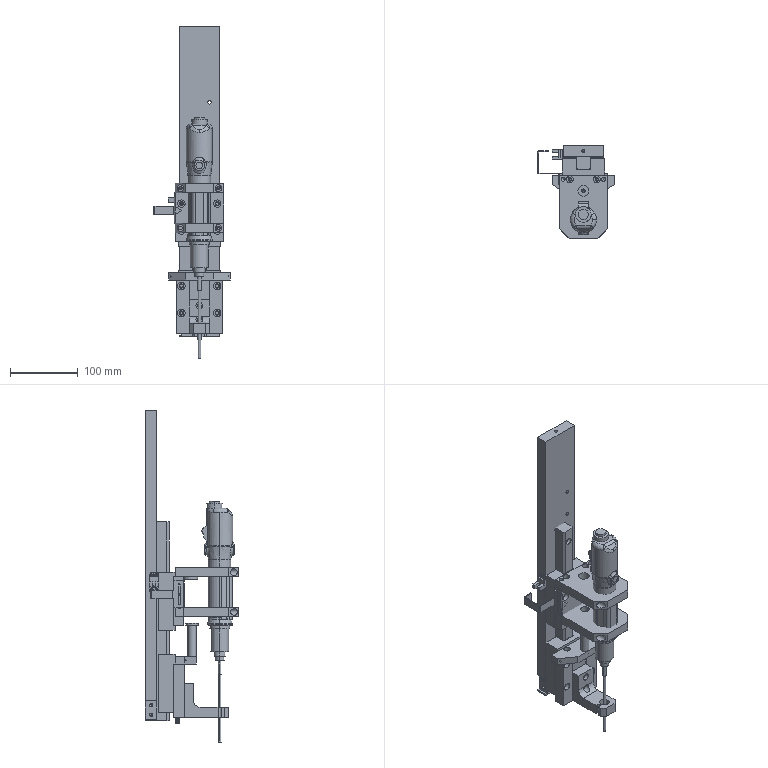Part | NX | 18 solids | 671 faces | box 112.8 x 138 x 491.298 mm | volume 1337292 mm3 | cylinder 291 | plane 275 | cone 68 | spline 21 | torus 14 | sphere 2 | commonest cylinder face diameters 6 x89 4.2 x28 10 x21 5.3 x17 5 x16 2.5 x13